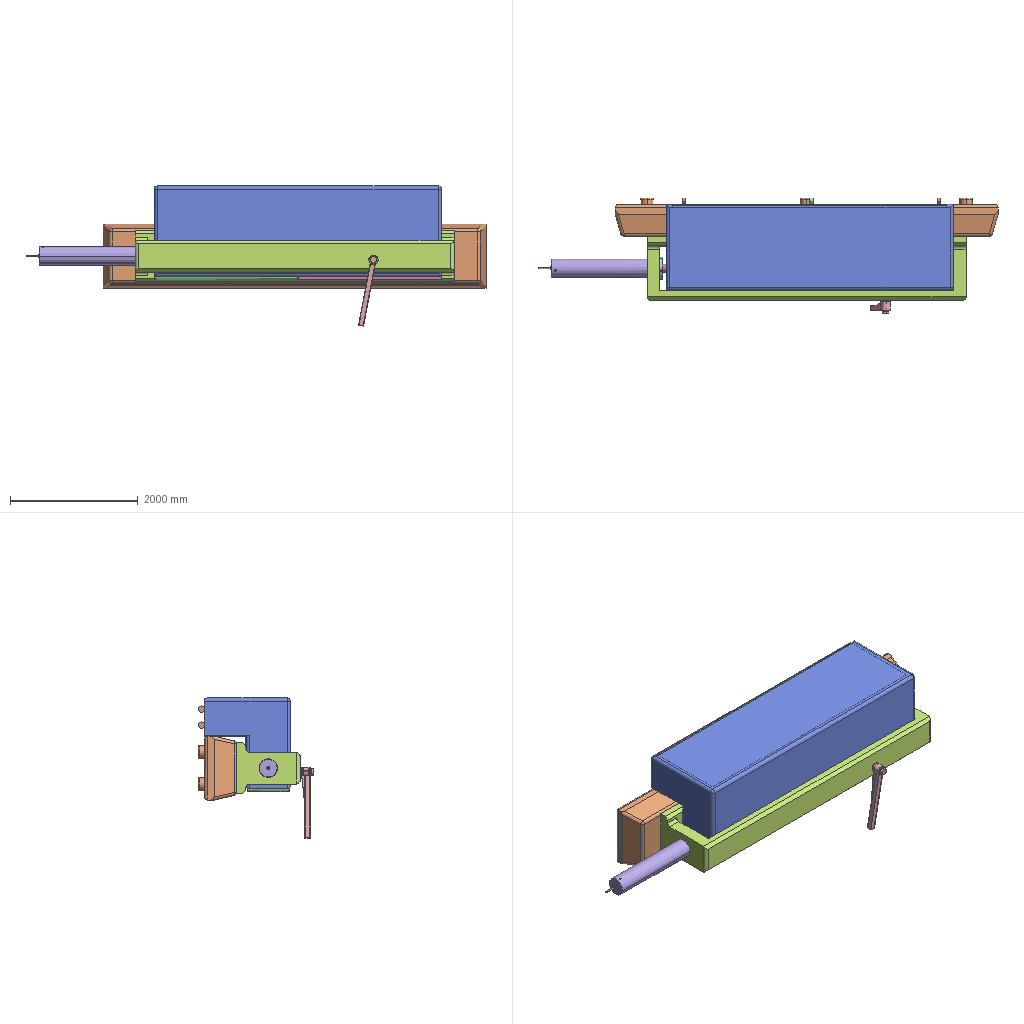Assembly | SolidWorks | 31 different items | 37 placed | box 7211 x 1815 x 2195 mm
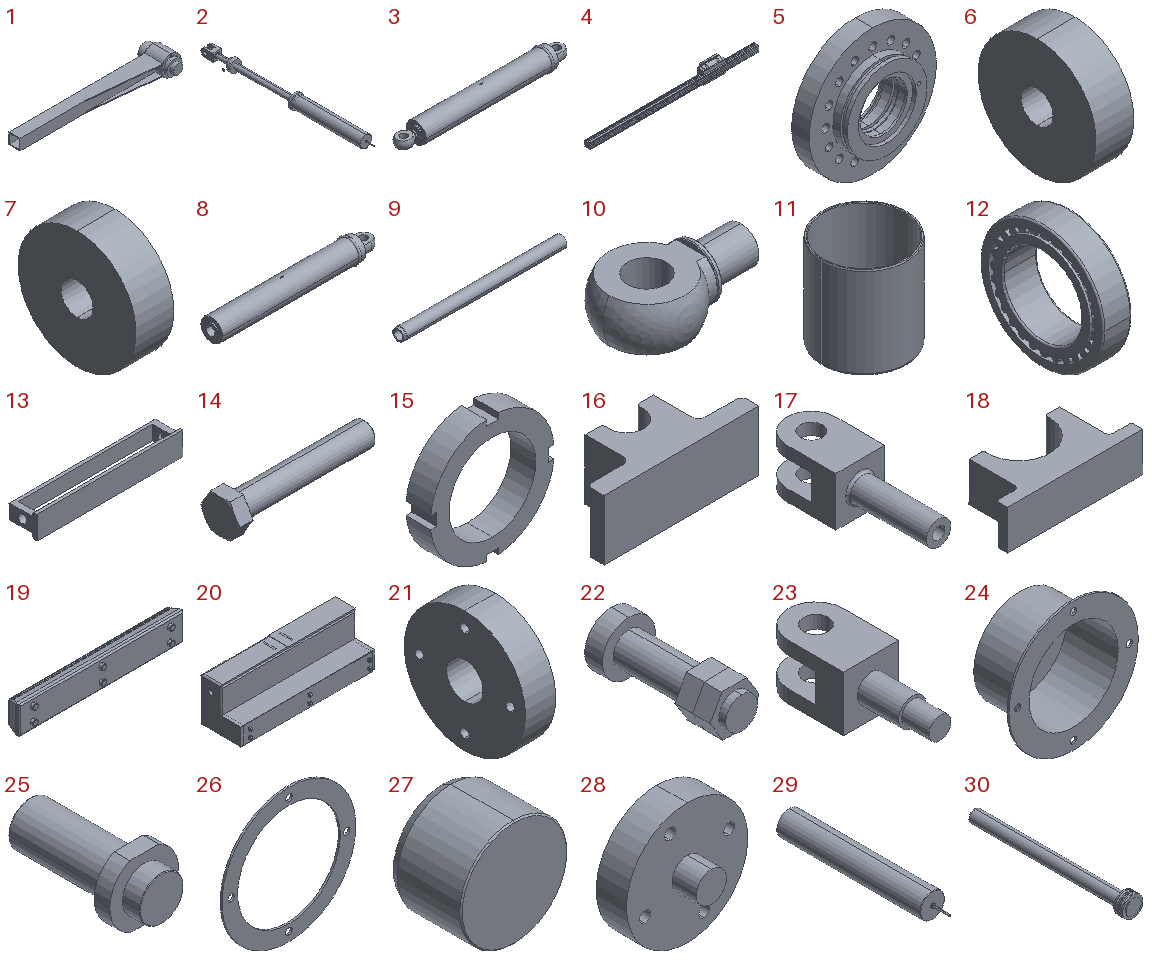Parts list (item | name | quantity | parent item | size | volume | features):
1 | (subassembly) | x1 | - | 1123 x 243 x 145 mm | 4299849 mm3 | features CompositeCurve 16
2 | (subassembly) | x1 | - | 424.619 x 4179 x 350 mm | 96090471 mm3 | features AEMSimFeature 1
3 | (subassembly) | x1 | - | 2283 x 316.65 x 300.3 mm | 112052939 mm3 | -
4 | (subassembly) | x2 | - | 1725 x 90 x 170 mm | 6825649 mm3 | -
5 | - | x1 | in 2 | 350 x 88 x 350 mm | 4363937 mm3 | features HoleWzd 4, 3DProfileFeature 1, RefAxis 1, Revolution 1
6 | - | x1 | - | 90 x 280 x 280 mm | 5133488 mm3 | features Revolution 1
7 | - | x1 | in 2 | 90 x 280 x 280 mm | 5133488 mm3 | features Revolution 1
8 | - | x1 | in 3 | 2027 x 316.65 x 300.3 mm | 94983659 mm3 | features BaseBody 1
9 | - | x1 | in 3 | 1535 x 110 x 110 mm | 13745437 mm3 | features BaseBody 1
10 | - | x1 | in 3 | 322 x 204 x 122.4 mm | 3250841 mm3 | features BaseBody 1
11 | - | x1 | in 3 | 94.981 x 95 x 102 mm | 72973 mm3 | features BaseBody 1
12 | - | x2 | in 1 | 31 x 110 x 110 mm | 131745 mm3 | features Revolution 3, CirPattern 1
13 | - | x1 | - | 5000 x 1000 x 800 mm | 1070403912 mm3 | features ICE 4, Attribute 2, Fillet 2, Chamfer 1, Extrusion 1, WeldmentFeature 1
14 | - | x4 | in 2 | 100.18 x 27.332 x 23.67 mm | 22963 mm3 | features RevCut 3, Boss 1, Chamfer 1, Extrusion 1, Fillet 1, LPattern 1
15 | - | x1 | in 1 | 99.499 x 20 x 99.499 mm | 76177 mm3 | features Extrusion 1
16 | - | x1 | - | 450 x 180.5 x 175 mm | 7476887 mm3 | features Fillet 2, Chamfer 1, Extrusion 1, ICE 1, MoveFace 1
17 | - | x1 | in 2 | 200 x 620 x 200 mm | 9111860 mm3 | features ICE 3, Extrusion 1, Fillet 1
18 | - | x1 | - | 600 x 270 x 175 mm | 14579348 mm3 | features Fillet 2, Chamfer 1, Extrusion 1, ICE 1, MoveFace 1
19 | - | x1 | - | 6000 x 600 x 1000 mm | 2807650462 mm3 | features ICE 5, Attribute 2, Fillet 2, Extrusion 1, WeldmentFeature 1
20 | - | x1 | - | 4500 x 1450 x 1471 mm | 1463085878 mm3 | features ICE 13, Cut 2, Fillet 2, LPattern 2, Extrusion 1
21 | - | x1 | in 2 | 50 x 200 x 200 mm | 1398637 mm3 | features 3DProfileFeature 1, CirPattern 1, HoleWzd 1, Revolution 1
22 | - | x2 | - | 150 x 370 x 150 mm | 3530229 mm3 | features ICE 1, LPattern 1, Revolution 1
23 | - | x1 | - | 200 x 550 x 200 mm | 8468645 mm3 | features ICE 4, Extrusion 1
24 | - | x1 | in 1 | 145 x 60 x 145 mm | 69889 mm3 | features CirPattern 1, ICE 1, Revolution 1
25 | - | x1 | in 1 | 110 x 210 x 100 mm | 941619 mm3 | features ICE 1, Revolution 1
26 | - | x1 | in 1 | 145 x 2 x 145 mm | 13364 mm3 | features CirPattern 1, Extrusion 1, ICE 1
27 | - | x1 | in 2 | 40 x 26.8 x 40 mm | 33387 mm3 | features Chamfer 2, Revolution 1
28 | - | x1 | in 2 | 200 x 95 x 200 mm | 1612580 mm3 | features Chamfer 1, HoleWzd 1, Revolution 1
29 | - | x1 | in 2 | 290 x 1911 x 290 mm | 49235613 mm3 | features HoleWzd 3, ICE 2, 3DProfileFeature 1, Revolution 1
30 | - | x1 | in 2 | 220 x 1728 x 220 mm | 25109118 mm3 | features Revolution 1
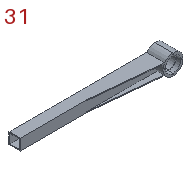31 | - | x1 | in 1 | 1122 x 130 x 145 mm | 2935310 mm3 | features CirPattern 2, HoleWzd 2, ICE 2, MirrorPattern 1, Revolution 1, Shell 1
Mates (type | each side: item.copy, entity, surface, feature):
In the top assembly
Symmetric | 13.1 face plane Boss-Extrude1 | 13.1 face plane Boss-Extrude1 | assembly plane | 3 times
Coincident | 13.1 face plane Cut-Extrude1 | 20.1 face plane Boss-Extrude1 | 2 times
Coincident | 13.1 face plane Boss-Extrude1 | 19.1 face plane Boss-Extrude1
Concentric | 13.1 face cylinder Cut-Extrude3 | 6.1 face cylinder Revolve1
Coincident | 13.1 face plane Cut-Extrude3 | 6.1 face plane Revolve1
Concentric | 13.1 face cylinder Cut-Extrude2 | 29.1 face cylinder Revolve1
Coincident | 13.1 face plane Cut-Extrude1 | 5.1 face plane Revolve1
Concentric | 10.1 face cylinder cylinder_hsg-k01-220_110_1500-g1401l1w | 17.1 face cylinder Boss-Extrude2
Concentric | 16.1 face cylinder Boss-Extrude1 | 17.1 face cylinder Boss-Extrude3
DistanceDim | 16.1 face plane Boss-Extrude1 | 17.1 face plane Boss-Extrude2
Width | 19.1 face plane Boss-Extrude1 | 19.1 face plane Boss-Extrude1 | 13.1 face plane Boss-Extrude1 | 13.1 face plane Boss-Extrude1
Coincident | 16.1 face plane Boss-Extrude1 | 17.1 face plane Boss-Extrude2
Concentric | 17.1 face cylinder Boss-Extrude2 | 22.1 face cylinder Revolve1
Coincident | 17.1 face plane Boss-Extrude2 | 22.1 face plane Revolve1
Width | 17.1 face plane Boss-Extrude2 | 17.1 face plane Boss-Extrude2 | 10.1 face plane cylinder_hsg-k01-220_110_1500-g1401l1w | 10.1 face plane cylinder_hsg-k01-220_110_1500-g1401l1w
Concentric | 8.1 face cylinder cylinder_hsg-k01-220_110_1500-g1401l1w | 30.1 face cylinder Revolve1
Concentric | 30.1 face cylinder Revolve1 | 23.1 face cylinder Boss-Extrude3
Concentric | 11.1 face cylinder cylinder_hsg-k01-220_110_1500-g1401l1w | 23.1 face cylinder Boss-Extrude2
Concentric | 30.1 face cylinder Revolve1 | 18.1 face cylinder Boss-Extrude1
DistanceDim | 18.1 face plane Boss-Extrude1 | 13.1 face plane Cut-Extrude1
Coincident | 20.1 face plane Boss-Extrude8 | 19.1 face plane Boss-Extrude1
Concentric | 23.1 face cylinder Boss-Extrude2 | 22.2 face cylinder Revolve1
Coincident | 23.1 face plane Boss-Extrude2 | 22.2 face plane Revolve1
Width | 19.1 face plane Boss-Extrude1 | 19.1 face plane Boss-Extrude1 | 13.1 face plane Boss-Extrude2 | 13.1 face plane Boss-Extrude2
Coincident | 13.1 face plane Boss-Extrude1 | 25.1 face plane Revolve1
In subassembly 1
Coincident | 31.1 plane | 1.1 plane | 3 times
Concentric | 31.1 edge | 12.1 edge
Coincident | 31.1 face plane Revolve1 | 12.1 face plane Revolve1
Concentric | 31.1 edge | 26.1 edge
Coincident | 12.1 face plane Revolve1 | 26.1 face plane Boss-Extrude1
Concentric | 31.1 edge | 12.2 edge
Coincident | 31.1 face plane Revolve1 | 12.2 face plane Revolve1
Concentric | 31.1 edge | 25.2 edge
Coincident | 12.1 face plane Revolve1 | 25.2 face plane Revolve1
Concentric | 25.2 edge | 15.1 edge
Coincident | 12.2 face plane Revolve1 | 15.1 face plane Boss-Extrude1
Concentric | 15.1 edge | 24.1 edge
Concentric | 31.1 edge | 24.1 edge | 2 times
Coincident | 31.1 face plane Revolve1 | 24.1 face plane Revolve1
In subassembly 2
Concentric | 29.2 face cylinder Revolve1 | 30.2 face cylinder Revolve1
Coincident | 30.2 plane | 2.1 plane
Coincident | 29.2 face plane Revolve1 | 5.2 face plane Revolve1
Concentric | 29.2 face cylinder Revolve1 | 5.2 face cylinder Revolve1
Coincident | 29.2 plane | 5.2 plane
Coincident | 30.2 face plane Revolve1 | 27.1 face plane Revolve1
Coincident | 27.1 plane | 2.1 plane
Concentric | 7.1 face cylinder Revolve1 | 28.1 face cylinder Revolve1
Coincident | 7.1 face plane Revolve1 | 28.1 face plane Revolve1
LimitDistanceDim | 30.2 face plane Revolve1 | 29.2 face plane Revolve1
Concentric | 28.1 face cylinder Revolve1 | 17.2 face cylinder Boss-Extrude3
Coincident | 28.1 face plane Revolve1 | 17.2 face plane Boss-Extrude3
Concentric | 30.2 face cylinder Revolve1 | 21.1 face cylinder Revolve1
Coincident | 30.2 face plane Revolve1 | 21.1 face plane Revolve1
Concentric | 28.1 face cylinder Revolve1 | 21.1 face cylinder Revolve1
Coincident | 28.1 face plane Revolve1 | 21.1 face plane Revolve1
Concentric | 28.1 face cylinder Ø18.0 (18) Diameter Hole1 | 14.1 face cylinder BaseBody
Coincident | 28.1 face plane Revolve1 | 14.1 face plane BaseHead
Concentric | 28.1 face cylinder Ø18.0 (18) Diameter Hole1 | 14.2 face cylinder BaseBody
Coincident | 28.1 face plane Revolve1 | 14.2 face plane BaseHead
Concentric | 28.1 face cylinder Ø18.0 (18) Diameter Hole1 | 14.3 face cylinder BaseBody
Coincident | 28.1 face plane Revolve1 | 14.3 face plane BaseHead
Concentric | 28.1 face cylinder Ø18.0 (18) Diameter Hole1 | 14.4 face cylinder BaseBody
Coincident | 28.1 face plane Revolve1 | 14.4 face plane BaseHead
In subassembly 3
Concentric | 8.2 face cylinder cylinder_hsg-k01-220_110_1500-g1401l1w | 9.1 face cylinder cylinder_hsg-k01-220_110_1500-g1401l1w
Concentric | 9.1 face cylinder cylinder_hsg-k01-220_110_1500-g1401l1w | 10.2 face cylinder cylinder_hsg-k01-220_110_1500-g1401l1w
Coincident | 9.1 face plane cylinder_hsg-k01-220_110_1500-g1401l1w | 10.2 face plane cylinder_hsg-k01-220_110_1500-g1401l1w
LimitDistanceDim | 9.1 face plane cylinder_hsg-k01-220_110_1500-g1401l1w | 8.2 face plane cylinder_hsg-k01-220_110_1500-g1401l1w